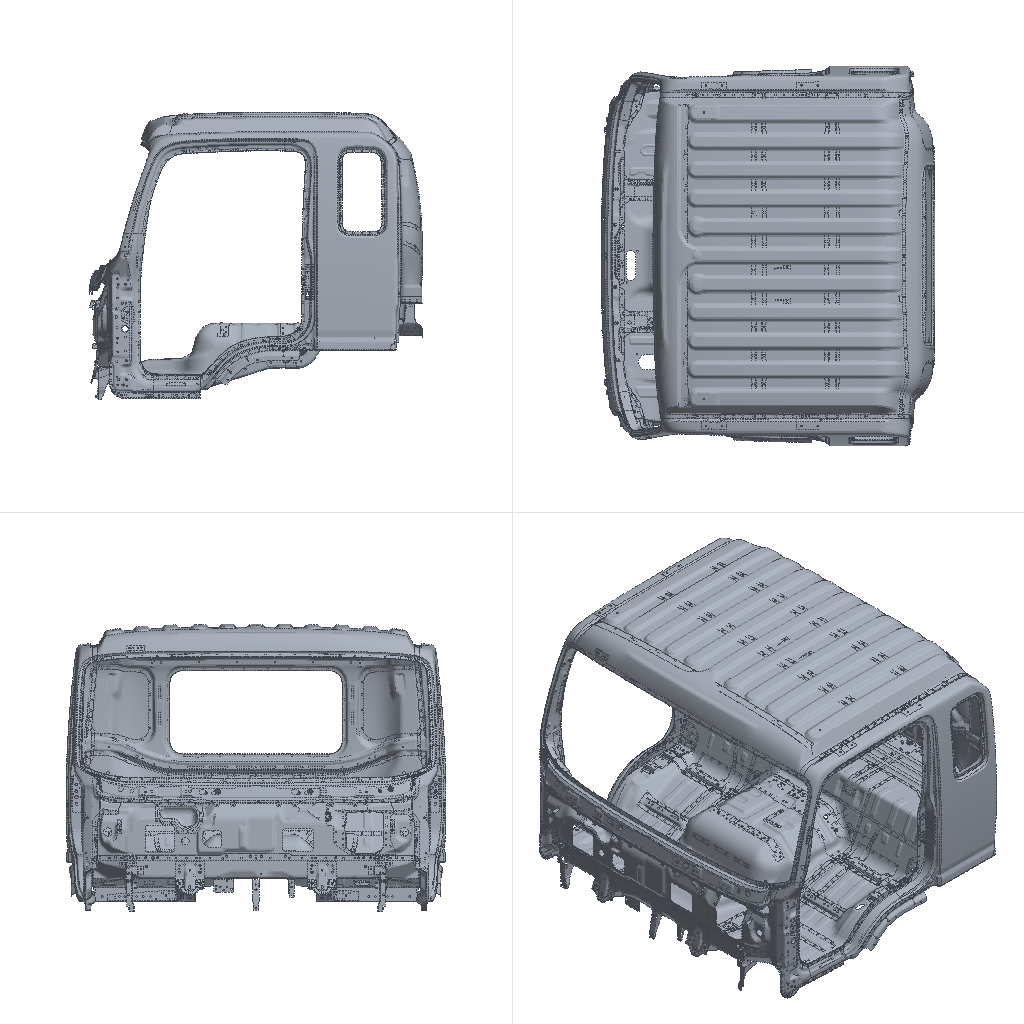Simulation study | nastran
Set-up summary:
category,name,step,type,value,unit,region
solver,nx_nastran
units,not stated in the deck,,not stated
analysis,deck,,static,static
analysis,solution,,SOL,101
load_step,SUBCASE 1,1,SUBCASE,SPC=1 LOAD=2
load_step,SUBCASE 2,2,SUBCASE,SPC=1 LOAD=3
load_step,SUBCASE 3,3,SUBCASE,SPC=1 LOAD=4
load_step,SUBCASE 4,4,SUBCASE,SPC=1 LOAD=5
load_step,requested,,,4
mesh,nodes,,,354455
mesh,elements,,,326452
element_type,CHEXA,,unverified,2286
element_type,CONM2,,mass,5
element_type,CQUAD4,,shell,313057
element_type,CTRIA3,,shell,13390
load,load commands in deck,,count,4
bc,support commands in deck,,count,4
check,setup vs results,,match,"every grid point's frame and coordinates and every element id; grid points of CHEXA, CQUAD4, CTRIA3 elements"
Nastran input file, long lists of numbers shortened:
$$------------------------------------------------------------------------------$
$$                                                                              $
$$ NASTRAN Input Deck Generated by HyperMesh Version  : 9.0b121                 $
$$ Generated using HyperMesh-Nastran Template Version : 9.0b121
$$                                                                              $
$$   Template:  general                                                         $
$$                                                                              $
$$------------------------------------------------------------------------------$
$$------------------------------------------------------------------------------$
$$                      Executive Control Cards                                 $
$$------------------------------------------------------------------------------$
SOL 101
CEND
$$------------------------------------------------------------------------------$
$$                      Case Control Cards                                      $
$$------------------------------------------------------------------------------$
  DISPLACEMENT(PLOT) = ALL
  STRESS(PLOT) = ALL
$
$HMNAME LOADSTEP               1"qudong"
SUBCASE       1
  LABEL=         qudong
  SPC =        1
  LOAD =        2
$
$HMNAME LOADSTEP               2"zhidong"
SUBCASE       2
  LABEL=         zhidong
  SPC =        1
  LOAD =        3
$
$HMNAME LOADSTEP               3"zhuanxiang"
SUBCASE       3
  LABEL=         zhuanxiang
  SPC =        1
  LOAD =        4
$
$HMNAME LOADSTEP               4"chuizhichongji"
SUBCASE       4
  LABEL=         chuizhichongji
  SPC =        1
  LOAD =        5
$$------------------------------------------------------------------------------$
$$                      Bulk Data Cards                                         $
$$------------------------------------------------------------------------------$
BEGIN BULK
PARAM,BAILOUT,-1
PARAM,POST,-1
$$
$$  GRID Data
$$
GRID           3        -862.084668.42731608.46
GRID           4        -860.106668.45771612.594
$ (354453 more lines like these left out)
$$
$$  SPOINT Data
$$
$
$  CONM2 Elements
$
CONM2    103453584122188       00.02692 0.0     0.0     0.0
CONM2    103453684122187       00.01172 0.0     0.0     0.0
CONM2    1034537 3777742       00.03968 0.0     0.0     0.0
CONM2    1034538 3777743       00.03765 0.0     0.0     0.0
CONM2    103453984121617       00.00412 0.0     0.0     0.0
$
$HMMOVE 84022690
$        1034535THRU     1034539
$
$$
$$------------------------------------------------------------------------------$
$$             Group Definitions                                                $
$$------------------------------------------------------------------------------$
$
$ RBE2 Elements - Single dependent node
$
RBE2      346590 3663307  123456 3657894
RBE2      346592 3663309  123456 3657892
$ (23 more lines like these left out)
$
$HMMOVE 57005014
$         346590  346592THRU      346597  346600THRU      346603  346605THRU
$         346608  346610THRU      346612  346614THRU      346620
$
$$
$$ RBE2 Elements - Multiple dependent nodes
$$
RBE2      346588 3663313  123456 3658184 3658185
RBE2      346589 3663312  123456 3657889 3658186
$ (313 more lines like these left out)
$
$HMMOVE 57005014
$         346588THRU      346589  346591  346598THRU      346599  346604  346609
$         346613  346621  346623THRU      346634  346869THRU      346871  346920
$       THRU      346924 1034533THRU     1034534 1033989
$
$
$  RBE3 Elements
$
RBE3     1045507        84122191  1234560.466386     123   288350.395963+
+            123   288750.063205     123   288740.074446     123   28834
RBE3     1045508        84122192  1234560.379884     123   288360.360056+
+            123   288640.126545     123   288750.133514     123   28835
$ (36572 more lines like these left out)
$
$HMMOVE 84022693
$        1045507THRU     1045510 1045512THRU     1045519 1045521THRU     1045528
$        1045530THRU     1045537 1045539THRU     1045546 1045548THRU     1045555
$ (765 more lines like these left out)
CTRIA3    144065       1   56012   56013   56011
CTRIA3    144068       1   56013   56014   56018
$ (13388 more lines like these left out)
$
$HMMOVE       14
$         144065  144068  144074  144076  144081  144146  144168  144188  144195
$         144200  144204  144221  144229  144299  144325  144329  144340  144574
$ (1233 more lines like these left out)
CQUAD4    159256       1   73815   73810   73807   73811
CQUAD4    159257       1   73811   73806   73812   73816
$ (313055 more lines like these left out)
$
$HMMOVE       14
$         159256THRU      159285  159287THRU      159294  159296THRU      159299
$         159301THRU      159306  159308THRU      159317  159320THRU      159326
$ (3543 more lines like these left out)
CHEXA    1045511      10841221918412219284122193841221948412219584122196+
+       8412219784122198
CHEXA    1045520      10841222018412220484122203841222028412220584122208+
+       8412220784122206
$ (4568 more lines like these left out)
$
$HMMOVE 84022692
$        1045511 1045520 1045529 1045538 1045547 1045556 1045565 1045574 1045583
$        1045592 1045601 1045610 1045619 1045628 1045637 1045646 1045655 1045664
$ (665 more lines like these left out)
PSHELL         8       11.6            1               1
$
$HMNAME PROP                   7"200" 4
$HWCOLOR PROP                  7       3
PSHELL         7       12.0            1               1
$
$HMNAME PROP                   6"250" 4
$HWCOLOR PROP                  6       3
PSHELL         6       12.5            1               1
$
$HMNAME PROP                   5"150" 4
$HWCOLOR PROP                  5       3
PSHELL         5       11.5            1               1
$
$HMNAME PROP                   4"100" 4
$HWCOLOR PROP                  4       3
PSHELL         4       11.0            1               1
$
$HMNAME PROP                   3"180" 4
$HWCOLOR PROP                  3       3
PSHELL         3       11.8            1               1
$
$HMNAME PROP                   2"120" 4
$HWCOLOR PROP                  2       3
PSHELL         2       11.2            1               1
$
$
$
$HMNAME PROP                   1"80" 4
$HWCOLOR PROP                  1       3
PSHELL         1       10.8            1               1
$$
$$  PSOLID Data
$
$HMNAME PROP                  10"spot" 5
$HWCOLOR PROP                 10       3
PSOLID        10       1
$$
$$------------------------------------------------------------------------------$
$$                      Material Definition Cards                               $
$$------------------------------------------------------------------------------$
$$--------------------------------------------------------------
$$ HYPERMESH TAGS
$$--------------------------------------------------------------
$$BEGIN TAGS
$$END TAGS
$$
$$  MAT1 Data
$
$HMNAME MAT                    1"steel" "MAT1"
$HWCOLOR MAT                   1       3
MAT1           1210000.0        0.3     1.60E-08
$$
$$
$$
$$------------------------------------------------------------------------------$
$ (29 more lines like these left out)
GRAV           2        9800.0  1.0     0.0     -1.0
$$
$HMNAME LOADCOL                3"zhidong"
$HWCOLOR LOADCOL               3       4
GRAV           3        9800.0  -1.0    0.0     -1.0
$$
$HMNAME LOADCOL                4"zhuanxiang"
$HWCOLOR LOADCOL               4       5
GRAV           4        9800.0  0.0     1.0     -1.0
$$
$HMNAME LOADCOL                5"chuizhichongji"
$HWCOLOR LOADCOL               5       6
GRAV           5        9800.0  0.0     0.0     3.0
$$
$$
$$
$$
$$
$$
$$
$$
$$
$$
$$
$$  SPC Data
$$
SPC            1 3777741  123   0.0
SPC            1 3777740  123   0.0
SPC            1 3777727  123   0.0
SPC            1 3777739  123   0.0
$HMASSEM 5400100       7 sidebody_L
$HMASSEM_IDS    5400101054005010540070105400303054007020540030205400102054001030
$HMASSEM_IDS    540011105400112054001210540030105400502054007080
$HMASSEM 5400200       6 sidebody_R
$HMASSEM_IDS    5400203054002110540021205400221054004010540040205400403054006010
$HMASSEM_IDS    540020405400602054008010540020105400204154001220
$HMASSEM 5700100       5 5700100
$HMASSEM_IDS    570010105700311057002010570032105700401057005010
$HMASSEM      28       4 5300010
$HMASSEM_IDS          16      17      18      19      20      21      22      24
$HMASSEM_IDS          25      26
$HMASSEM      27       3 5600010
$HMASSEM_IDS          14      15
$HMASSEM       1       3 REAR_FLOOR
$HMASSEM_IDS    5100993051009900510030105100311051003610510037105100331051003210
$HMASSEM_IDS    5100181051000410510002105100761051007510510074105100791051007520
$HMASSEM_IDS    5100481051001110510085105100852051007411510068105100131051005210
$HMASSEM_IDS    5100121051005211510055105100141051009911510017105100181251009310
$HMASSEM_IDS    5100451051004210510048115100431151004610510041105100211051004410
$HMASSEM_IDS    5100601051009710510099405100271051002410510023105100621051002210
$HMASSEM_IDS    5100621151004710510045115100561351005410510064105100701051008010
$HMASSEM_IDS    5100721051008210510071105100561051005611510056125100431051005311
$HMASSEM_IDS    5100031051000311510059105100691051005710510067105100102151001020
$HMASSEM_IDS    5100501051009410510077105100991051003410510078105100971151001811
$
ENDDATA
Results summary:
result,analysis,,,static
result,last_loadstep,,,4
result,primary field,,,displacements
result,max displacement,,,2.309,model units